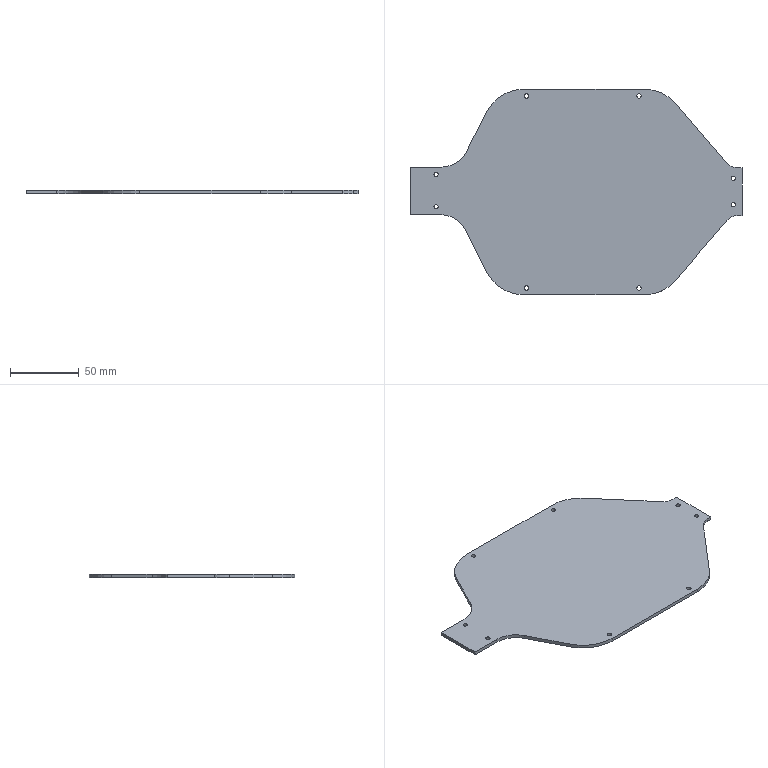Part | STEP file | Dodanie-wyci_gni_cie2_3 | 1 solid | 30 faces | box 242.308 x 150 x 2.5 mm | volume 66669 mm3 | cylinder 16 | plane 14 | commonest cylinder face diameters 3.16 x4 60 x4 3 x2 3.05 x2 20 x2 40 x2